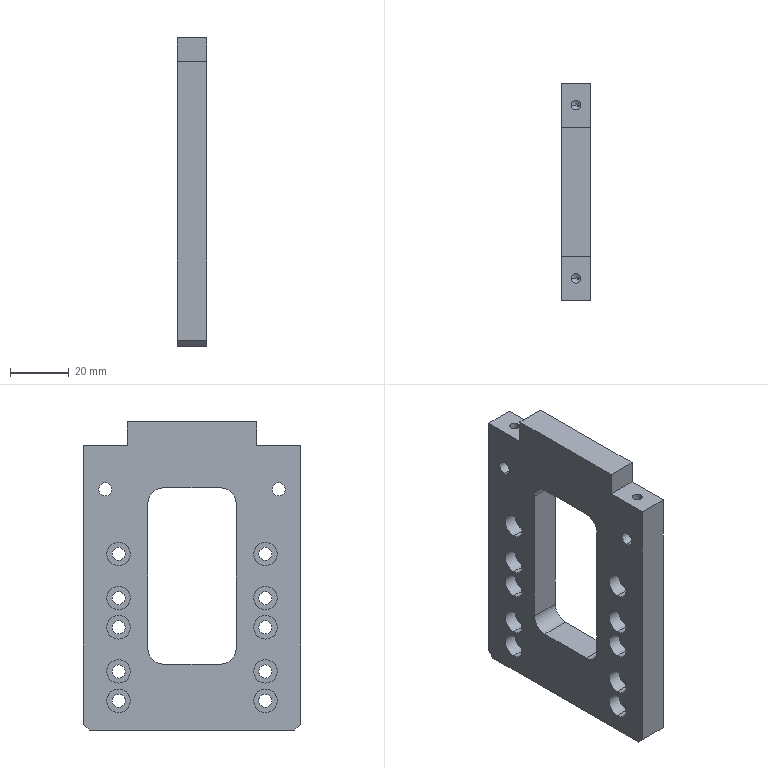Part | SolidWorks | features HoleWzd 4, Cut 2, MoveFace 2, Chamfer 1, DelFace 1, Extrusion 1, ICE 1 | 1 solid | 88 faces | box 10 x 74 x 105 mm | volume 53491 mm3 | cylinder 56 | plane 28 | cone 4 | commonest cylinder face diameters 4.5 x24 8 x24 3.3 x4 10 x4